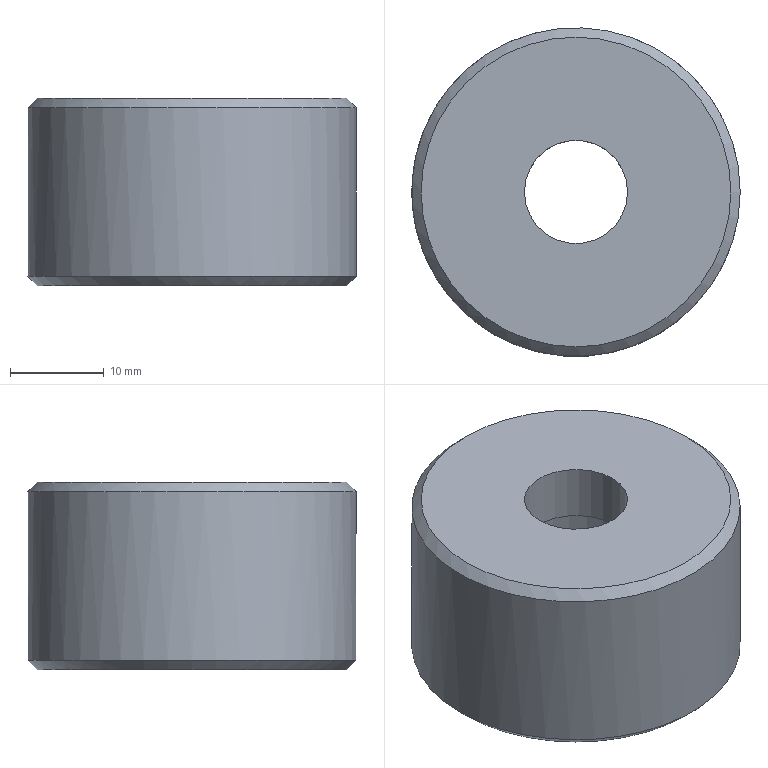Part | NX | features solid 2 | 1 solid | 8 faces | box 35 x 35 x 20 mm | volume 15386 mm3 | plane 3 | cylinder 3 | cone 2 | commonest cylinder face diameters 11 x1 17 x1 35 x1
STEP:
#1=CARTESIAN_POINT('',(1599.142,27.009,29.999));
#2=VERTEX_POINT('',#1);
#3=CARTESIAN_POINT('',(1582.642,27.009,29.999));
#4=DIRECTION('',(0.,0.,1.));
#5=DIRECTION('',(1.,0.,0.));
#6=AXIS2_PLACEMENT_3D('',#3,#4,#5);
#7=CIRCLE('',#6,16.5);
#8=EDGE_CURVE('',#2,#2,#7,.F.);
#9=ORIENTED_EDGE('',*,*,#8,.T.);
#10=EDGE_LOOP('',(#9));
#11=FACE_BOUND('',#10,.T.);
#12=CARTESIAN_POINT('',(1591.142,27.009,29.999));
#13=VERTEX_POINT('',#12);
#14=CARTESIAN_POINT('',(1582.642,27.009,29.999));
#15=DIRECTION('',(0.,0.,1.));
#16=DIRECTION('',(1.,0.,0.));
#17=AXIS2_PLACEMENT_3D('',#14,#15,#16);
#18=CIRCLE('',#17,8.5);
#19=EDGE_CURVE('',#13,#13,#18,.T.);
#20=ORIENTED_EDGE('',*,*,#19,.T.);
#21=EDGE_LOOP('',(#20));
#22=FACE_BOUND('',#21,.T.);
#23=CARTESIAN_POINT('',(1554.955,6.94,29.999));
#24=DIRECTION('',(0.,0.,1.));
#25=DIRECTION('',(-1.,0.,0.));
#26=AXIS2_PLACEMENT_3D('',#23,#24,#25);
#27=PLANE('',#26);
#28=ADVANCED_FACE('',(#11,#22),#27,.F.);
#29=CARTESIAN_POINT('',(1599.142,27.009,49.999));
#30=VERTEX_POINT('',#29);
#31=CARTESIAN_POINT('',(1582.642,27.009,49.999));
#32=DIRECTION('',(0.,0.,1.));
#33=DIRECTION('',(1.,0.,0.));
#34=AXIS2_PLACEMENT_3D('',#31,#32,#33);
#35=CIRCLE('',#34,16.5);
#36=EDGE_CURVE('',#30,#30,#35,.T.);
#37=ORIENTED_EDGE('',*,*,#36,.T.);
#38=EDGE_LOOP('',(#37));
#39=FACE_BOUND('',#38,.T.);
#40=CARTESIAN_POINT('',(1588.142,27.009,49.999));
#41=VERTEX_POINT('',#40);
#42=CARTESIAN_POINT('',(1582.642,27.009,49.999));
#43=DIRECTION('',(0.,0.,1.));
#44=DIRECTION('',(1.,0.,0.));
#45=AXIS2_PLACEMENT_3D('',#42,#43,#44);
#46=CIRCLE('',#45,5.5);
#47=EDGE_CURVE('',#41,#41,#46,.T.);
#48=ORIENTED_EDGE('',*,*,#47,.F.);
#49=EDGE_LOOP('',(#48));
#50=FACE_BOUND('',#49,.T.);
#51=CARTESIAN_POINT('',(1582.642,27.009,49.999));
#52=DIRECTION('',(0.,0.,1.));
#53=DIRECTION('',(1.,0.,0.));
#54=AXIS2_PLACEMENT_3D('',#51,#52,#53);
#55=PLANE('',#54);
#56=ADVANCED_FACE('',(#39,#50),#55,.T.);
#57=CARTESIAN_POINT('',(1600.142,27.009,48.999));
#58=VERTEX_POINT('',#57);
#59=CARTESIAN_POINT('',(1582.642,27.009,48.999));
#60=DIRECTION('',(0.,0.,1.));
#61=DIRECTION('',(1.,0.,0.));
#62=AXIS2_PLACEMENT_3D('',#59,#60,#61);
#63=CIRCLE('',#62,17.5);
#64=EDGE_CURVE('',#58,#58,#63,.F.);
#65=ORIENTED_EDGE('',*,*,#64,.T.);
#66=EDGE_LOOP('',(#65));
#67=FACE_BOUND('',#66,.T.);
#68=CARTESIAN_POINT('',(1565.142,27.009,30.999));
#69=VERTEX_POINT('',#68);
#70=CARTESIAN_POINT('',(1582.642,27.009,30.999));
#71=DIRECTION('',(0.,0.,-1.));
#72=DIRECTION('',(-1.,0.,0.));
#73=AXIS2_PLACEMENT_3D('',#70,#71,#72);
#74=CIRCLE('',#73,17.5);
#75=EDGE_CURVE('',#69,#69,#74,.F.);
#76=ORIENTED_EDGE('',*,*,#75,.T.);
#77=EDGE_LOOP('',(#76));
#78=FACE_BOUND('',#77,.T.);
#79=CARTESIAN_POINT('',(1582.642,27.009,49.999));
#80=DIRECTION('',(0.,0.,-1.));
#81=DIRECTION('',(1.,0.,0.));
#82=AXIS2_PLACEMENT_3D('',#79,#80,#81);
#83=CYLINDRICAL_SURFACE('',#82,17.5);
#84=ADVANCED_FACE('',(#67,#78),#83,.T.);
#85=ORIENTED_EDGE('',*,*,#47,.T.);
#86=EDGE_LOOP('',(#85));
#87=FACE_BOUND('',#86,.T.);
#88=CARTESIAN_POINT('',(1588.142,27.009,43.999));
#89=VERTEX_POINT('',#88);
#90=CARTESIAN_POINT('',(1582.642,27.009,43.999));
#91=DIRECTION('',(0.,0.,1.));
#92=DIRECTION('',(1.,0.,0.));
#93=AXIS2_PLACEMENT_3D('',#90,#91,#92);
#94=CIRCLE('',#93,5.5);
#95=EDGE_CURVE('',#89,#89,#94,.F.);
#96=ORIENTED_EDGE('',*,*,#95,.T.);
#97=EDGE_LOOP('',(#96));
#98=FACE_BOUND('',#97,.T.);
#99=CARTESIAN_POINT('',(1582.642,27.009,99.999));
#100=DIRECTION('',(0.,0.,1.));
#101=DIRECTION('',(1.,0.,0.));
#102=AXIS2_PLACEMENT_3D('',#99,#100,#101);
#103=CYLINDRICAL_SURFACE('',#102,5.5);
#104=ADVANCED_FACE('',(#87,#98),#103,.F.);
#105=ORIENTED_EDGE('',*,*,#95,.F.);
#106=EDGE_LOOP('',(#105));
#107=FACE_BOUND('',#106,.T.);
#108=CARTESIAN_POINT('',(1591.142,27.009,43.999));
#109=VERTEX_POINT('',#108);
#110=CARTESIAN_POINT('',(1582.642,27.009,43.999));
#111=DIRECTION('',(0.,0.,1.));
#112=DIRECTION('',(1.,0.,0.));
#113=AXIS2_PLACEMENT_3D('',#110,#111,#112);
#114=CIRCLE('',#113,8.5);
#115=EDGE_CURVE('',#109,#109,#114,.F.);
#116=ORIENTED_EDGE('',*,*,#115,.T.);
#117=EDGE_LOOP('',(#116));
#118=FACE_BOUND('',#117,.T.);
#119=CARTESIAN_POINT('',(1582.642,27.009,43.999));
#120=DIRECTION('',(0.,0.,1.));
#121=DIRECTION('',(1.,0.,0.));
#122=AXIS2_PLACEMENT_3D('',#119,#120,#121);
#123=PLANE('',#122);
#124=ADVANCED_FACE('',(#107,#118),#123,.F.);
#125=ORIENTED_EDGE('',*,*,#115,.F.);
#126=EDGE_LOOP('',(#125));
#127=FACE_BOUND('',#126,.T.);
#128=ORIENTED_EDGE('',*,*,#19,.F.);
#129=EDGE_LOOP('',(#128));
#130=FACE_BOUND('',#129,.T.);
#131=CARTESIAN_POINT('',(1582.642,27.009,-0.0008318));
#132=DIRECTION('',(0.,0.,1.));
#133=DIRECTION('',(1.,0.,0.));
#134=AXIS2_PLACEMENT_3D('',#131,#132,#133);
#135=CYLINDRICAL_SURFACE('',#134,8.5);
#136=ADVANCED_FACE('',(#127,#130),#135,.F.);
#137=ORIENTED_EDGE('',*,*,#36,.F.);
#138=EDGE_LOOP('',(#137));
#139=FACE_BOUND('',#138,.T.);
#140=ORIENTED_EDGE('',*,*,#64,.F.);
#141=EDGE_LOOP('',(#140));
#142=FACE_BOUND('',#141,.T.);
#143=CARTESIAN_POINT('',(1582.642,27.009,48.999));
#144=DIRECTION('',(0.,0.,-1.));
#145=DIRECTION('',(-1.,0.,0.));
#146=AXIS2_PLACEMENT_3D('',#143,#144,#145);
#147=CONICAL_SURFACE('',#146,17.5,0.7854);
#148=ADVANCED_FACE('',(#139,#142),#147,.T.);
#149=ORIENTED_EDGE('',*,*,#8,.F.);
#150=EDGE_LOOP('',(#149));
#151=FACE_BOUND('',#150,.T.);
#152=ORIENTED_EDGE('',*,*,#75,.F.);
#153=EDGE_LOOP('',(#152));
#154=FACE_BOUND('',#153,.T.);
#155=CARTESIAN_POINT('',(1582.642,27.009,30.999));
#156=DIRECTION('',(0.,0.,1.));
#157=DIRECTION('',(1.,0.,0.));
#158=AXIS2_PLACEMENT_3D('',#155,#156,#157);
#159=CONICAL_SURFACE('',#158,17.5,0.7854);
#160=ADVANCED_FACE('',(#151,#154),#159,.T.);
#161=CLOSED_SHELL('',(#28,#56,#84,#104,#124,#136,#148,#160));
#162=MANIFOLD_SOLID_BREP('',#161);
#163=(LENGTH_UNIT()NAMED_UNIT(*)SI_UNIT(.MILLI.,.METRE.));
#164=UNCERTAINTY_MEASURE_WITH_UNIT(LENGTH_MEASURE(0.00001),#163,'','');
#165=(NAMED_UNIT(*)PLANE_ANGLE_UNIT()SI_UNIT($,.RADIAN.));
#166=(NAMED_UNIT(*)SI_UNIT($,.STERADIAN.)SOLID_ANGLE_UNIT());
#167=(GEOMETRIC_REPRESENTATION_CONTEXT(3)GLOBAL_UNCERTAINTY_ASSIGNED_CONTEXT((#164))GLOBAL_UNIT_ASSIGNED_CONTEXT((#163,#165,#166))REPRESENTATION_CONTEXT('',''));
#168=ADVANCED_BREP_SHAPE_REPRESENTATION('',(#162),#167);